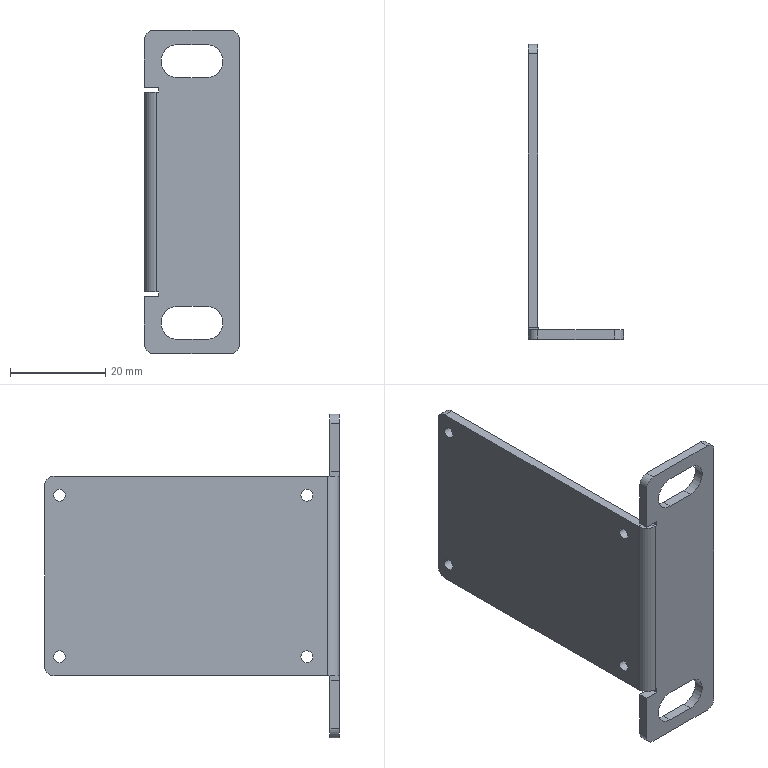Part | SolidWorks | features ICE 4, Cut 1, ExtruThin 1, Fillet 1, FlatPattern 1, FlattenBends 1, ProcessBends 1, SheetMetal 1 | 1 solid | 44 faces | box 20 x 62 x 68 mm | volume 7322 mm3 | plane 24 | cylinder 20 | commonest cylinder face diameters 2.5 x8 4 x6 7 x4 1 x1 5 x1
STEP:
#1=CARTESIAN_POINT('',(0.,8.1,17.));
#2=VERTEX_POINT('',#1);
#3=CARTESIAN_POINT('',(0.,5.6,17.));
#4=VERTEX_POINT('',#3);
#5=CARTESIAN_POINT('',(0.,6.85,17.));
#6=DIRECTION('',(-1.,0.,0.));
#7=DIRECTION('',(0.,-1.,0.));
#8=AXIS2_PLACEMENT_3D('',#5,#6,#7);
#9=CIRCLE('',#8,1.25);
#10=EDGE_CURVE('',#2,#4,#9,.T.);
#11=ORIENTED_EDGE('',*,*,#10,.T.);
#12=CARTESIAN_POINT('',(2.,5.6,17.));
#13=VERTEX_POINT('',#12);
#14=CARTESIAN_POINT('',(-8.,5.6,17.));
#15=DIRECTION('',(1.,0.,0.));
#16=VECTOR('',#15,1000.);
#17=LINE('',#14,#16);
#18=EDGE_CURVE('',#4,#13,#17,.T.);
#19=ORIENTED_EDGE('',*,*,#18,.T.);
#20=CARTESIAN_POINT('',(2.,8.1,17.));
#21=VERTEX_POINT('',#20);
#22=CARTESIAN_POINT('',(2.,6.85,17.));
#23=DIRECTION('',(1.,0.,0.));
#24=DIRECTION('',(0.,1.,0.));
#25=AXIS2_PLACEMENT_3D('',#22,#23,#24);
#26=CIRCLE('',#25,1.25);
#27=EDGE_CURVE('',#13,#21,#26,.T.);
#28=ORIENTED_EDGE('',*,*,#27,.T.);
#29=CARTESIAN_POINT('',(-8.,8.1,17.));
#30=DIRECTION('',(1.,0.,0.));
#31=VECTOR('',#30,1000.);
#32=LINE('',#29,#31);
#33=EDGE_CURVE('',#2,#21,#32,.T.);
#34=ORIENTED_EDGE('',*,*,#33,.F.);
#35=EDGE_LOOP('',(#11,#19,#28,#34));
#36=FACE_OUTER_BOUND('',#35,.T.);
#37=CARTESIAN_POINT('',(-8.,6.85,17.));
#38=DIRECTION('',(1.,0.,0.));
#39=DIRECTION('',(0.,1.,0.));
#40=AXIS2_PLACEMENT_3D('',#37,#38,#39);
#41=CYLINDRICAL_SURFACE('',#40,1.25);
#42=ADVANCED_FACE('',(#36),#41,.F.);
#43=CARTESIAN_POINT('',(0.,8.1,-17.));
#44=VERTEX_POINT('',#43);
#45=CARTESIAN_POINT('',(0.,5.6,-17.));
#46=VERTEX_POINT('',#45);
#47=CARTESIAN_POINT('',(0.,6.85,-17.));
#48=DIRECTION('',(-1.,0.,0.));
#49=DIRECTION('',(0.,-1.,0.));
#50=AXIS2_PLACEMENT_3D('',#47,#48,#49);
#51=CIRCLE('',#50,1.25);
#52=EDGE_CURVE('',#44,#46,#51,.T.);
#53=ORIENTED_EDGE('',*,*,#52,.T.);
#54=CARTESIAN_POINT('',(2.,5.6,-17.));
#55=VERTEX_POINT('',#54);
#56=CARTESIAN_POINT('',(-8.,5.6,-17.));
#57=DIRECTION('',(1.,0.,0.));
#58=VECTOR('',#57,1000.);
#59=LINE('',#56,#58);
#60=EDGE_CURVE('',#46,#55,#59,.T.);
#61=ORIENTED_EDGE('',*,*,#60,.T.);
#62=CARTESIAN_POINT('',(2.,8.1,-17.));
#63=VERTEX_POINT('',#62);
#64=CARTESIAN_POINT('',(2.,6.85,-17.));
#65=DIRECTION('',(1.,0.,0.));
#66=DIRECTION('',(0.,1.,0.));
#67=AXIS2_PLACEMENT_3D('',#64,#65,#66);
#68=CIRCLE('',#67,1.25);
#69=EDGE_CURVE('',#55,#63,#68,.T.);
#70=ORIENTED_EDGE('',*,*,#69,.T.);
#71=CARTESIAN_POINT('',(-8.,8.1,-17.));
#72=DIRECTION('',(1.,0.,0.));
#73=VECTOR('',#72,1000.);
#74=LINE('',#71,#73);
#75=EDGE_CURVE('',#44,#63,#74,.T.);
#76=ORIENTED_EDGE('',*,*,#75,.F.);
#77=EDGE_LOOP('',(#53,#61,#70,#76));
#78=FACE_OUTER_BOUND('',#77,.T.);
#79=CARTESIAN_POINT('',(-8.,6.85,-17.));
#80=DIRECTION('',(1.,0.,0.));
#81=DIRECTION('',(0.,1.,0.));
#82=AXIS2_PLACEMENT_3D('',#79,#80,#81);
#83=CYLINDRICAL_SURFACE('',#82,1.25);
#84=ADVANCED_FACE('',(#78),#83,.F.);
#85=CARTESIAN_POINT('',(0.,60.1,-17.));
#86=VERTEX_POINT('',#85);
#87=CARTESIAN_POINT('',(0.,57.6,-17.));
#88=VERTEX_POINT('',#87);
#89=CARTESIAN_POINT('',(0.,58.85,-17.));
#90=DIRECTION('',(-1.,0.,0.));
#91=DIRECTION('',(0.,-1.,0.));
#92=AXIS2_PLACEMENT_3D('',#89,#90,#91);
#93=CIRCLE('',#92,1.25);
#94=EDGE_CURVE('',#86,#88,#93,.T.);
#95=ORIENTED_EDGE('',*,*,#94,.T.);
#96=CARTESIAN_POINT('',(2.,57.6,-17.));
#97=VERTEX_POINT('',#96);
#98=CARTESIAN_POINT('',(-8.,57.6,-17.));
#99=DIRECTION('',(1.,0.,0.));
#100=VECTOR('',#99,1000.);
#101=LINE('',#98,#100);
#102=EDGE_CURVE('',#88,#97,#101,.T.);
#103=ORIENTED_EDGE('',*,*,#102,.T.);
#104=CARTESIAN_POINT('',(2.,60.1,-17.));
#105=VERTEX_POINT('',#104);
#106=CARTESIAN_POINT('',(2.,58.85,-17.));
#107=DIRECTION('',(1.,0.,0.));
#108=DIRECTION('',(0.,1.,0.));
#109=AXIS2_PLACEMENT_3D('',#106,#107,#108);
#110=CIRCLE('',#109,1.25);
#111=EDGE_CURVE('',#97,#105,#110,.T.);
#112=ORIENTED_EDGE('',*,*,#111,.T.);
#113=CARTESIAN_POINT('',(-8.,60.1,-17.));
#114=DIRECTION('',(1.,0.,0.));
#115=VECTOR('',#114,1000.);
#116=LINE('',#113,#115);
#117=EDGE_CURVE('',#86,#105,#116,.T.);
#118=ORIENTED_EDGE('',*,*,#117,.F.);
#119=EDGE_LOOP('',(#95,#103,#112,#118));
#120=FACE_OUTER_BOUND('',#119,.T.);
#121=CARTESIAN_POINT('',(-8.,58.85,-17.));
#122=DIRECTION('',(1.,0.,0.));
#123=DIRECTION('',(0.,1.,0.));
#124=AXIS2_PLACEMENT_3D('',#121,#122,#123);
#125=CYLINDRICAL_SURFACE('',#124,1.25);
#126=ADVANCED_FACE('',(#120),#125,.F.);
#127=CARTESIAN_POINT('',(0.,60.1,17.));
#128=VERTEX_POINT('',#127);
#129=CARTESIAN_POINT('',(0.,57.6,17.));
#130=VERTEX_POINT('',#129);
#131=CARTESIAN_POINT('',(0.,58.85,17.));
#132=DIRECTION('',(-1.,0.,0.));
#133=DIRECTION('',(0.,-1.,0.));
#134=AXIS2_PLACEMENT_3D('',#131,#132,#133);
#135=CIRCLE('',#134,1.25);
#136=EDGE_CURVE('',#128,#130,#135,.T.);
#137=ORIENTED_EDGE('',*,*,#136,.T.);
#138=CARTESIAN_POINT('',(2.,57.6,17.));
#139=VERTEX_POINT('',#138);
#140=CARTESIAN_POINT('',(-8.,57.6,17.));
#141=DIRECTION('',(1.,0.,0.));
#142=VECTOR('',#141,1000.);
#143=LINE('',#140,#142);
#144=EDGE_CURVE('',#130,#139,#143,.T.);
#145=ORIENTED_EDGE('',*,*,#144,.T.);
#146=CARTESIAN_POINT('',(2.,60.1,17.));
#147=VERTEX_POINT('',#146);
#148=CARTESIAN_POINT('',(2.,58.85,17.));
#149=DIRECTION('',(1.,0.,0.));
#150=DIRECTION('',(0.,1.,0.));
#151=AXIS2_PLACEMENT_3D('',#148,#149,#150);
#152=CIRCLE('',#151,1.25);
#153=EDGE_CURVE('',#139,#147,#152,.T.);
#154=ORIENTED_EDGE('',*,*,#153,.T.);
#155=CARTESIAN_POINT('',(-8.,60.1,17.));
#156=DIRECTION('',(1.,0.,0.));
#157=VECTOR('',#156,1000.);
#158=LINE('',#155,#157);
#159=EDGE_CURVE('',#128,#147,#158,.T.);
#160=ORIENTED_EDGE('',*,*,#159,.F.);
#161=EDGE_LOOP('',(#137,#145,#154,#160));
#162=FACE_OUTER_BOUND('',#161,.T.);
#163=CARTESIAN_POINT('',(-8.,58.85,17.));
#164=DIRECTION('',(1.,0.,0.));
#165=DIRECTION('',(0.,1.,0.));
#166=AXIS2_PLACEMENT_3D('',#163,#164,#165);
#167=CYLINDRICAL_SURFACE('',#166,1.25);
#168=ADVANCED_FACE('',(#162),#167,.F.);
#169=CARTESIAN_POINT('',(7.,0.,-31.));
#170=VERTEX_POINT('',#169);
#171=CARTESIAN_POINT('',(13.,0.,-31.));
#172=VERTEX_POINT('',#171);
#173=CARTESIAN_POINT('',(0.,0.,-31.));
#174=DIRECTION('',(1.,0.,0.));
#175=VECTOR('',#174,1000.);
#176=LINE('',#173,#175);
#177=EDGE_CURVE('',#170,#172,#176,.T.);
#178=ORIENTED_EDGE('',*,*,#177,.T.);
#179=CARTESIAN_POINT('',(13.,2.,-31.));
#180=VERTEX_POINT('',#179);
#181=CARTESIAN_POINT('',(13.,-1.,-31.));
#182=DIRECTION('',(0.,1.,0.));
#183=VECTOR('',#182,1000.);
#184=LINE('',#181,#183);
#185=EDGE_CURVE('',#172,#180,#184,.T.);
#186=ORIENTED_EDGE('',*,*,#185,.T.);
#187=CARTESIAN_POINT('',(7.,2.,-31.));
#188=VERTEX_POINT('',#187);
#189=CARTESIAN_POINT('',(7.,2.,-31.));
#190=DIRECTION('',(-1.,0.,0.));
#191=VECTOR('',#190,1000.);
#192=LINE('',#189,#191);
#193=EDGE_CURVE('',#180,#188,#192,.T.);
#194=ORIENTED_EDGE('',*,*,#193,.T.);
#195=CARTESIAN_POINT('',(7.,-1.,-31.));
#196=DIRECTION('',(0.,1.,0.));
#197=VECTOR('',#196,1000.);
#198=LINE('',#195,#197);
#199=EDGE_CURVE('',#170,#188,#198,.T.);
#200=ORIENTED_EDGE('',*,*,#199,.F.);
#201=EDGE_LOOP('',(#178,#186,#194,#200));
#202=FACE_OUTER_BOUND('',#201,.T.);
#203=CARTESIAN_POINT('',(7.,-1.,-31.));
#204=DIRECTION('',(0.,0.,-1.));
#205=DIRECTION('',(-1.,0.,0.));
#206=AXIS2_PLACEMENT_3D('',#203,#204,#205);
#207=PLANE('',#206);
#208=ADVANCED_FACE('',(#202),#207,.F.);
#209=CARTESIAN_POINT('',(13.,0.,-24.));
#210=VERTEX_POINT('',#209);
#211=CARTESIAN_POINT('',(13.,0.,-27.5));
#212=DIRECTION('',(0.,-1.,0.));
#213=DIRECTION('',(0.,0.,-1.));
#214=AXIS2_PLACEMENT_3D('',#211,#212,#213);
#215=CIRCLE('',#214,3.5);
#216=EDGE_CURVE('',#172,#210,#215,.T.);
#217=ORIENTED_EDGE('',*,*,#216,.T.);
#218=CARTESIAN_POINT('',(13.,2.,-24.));
#219=VERTEX_POINT('',#218);
#220=CARTESIAN_POINT('',(13.,-1.,-24.));
#221=DIRECTION('',(0.,1.,0.));
#222=VECTOR('',#221,1000.);
#223=LINE('',#220,#222);
#224=EDGE_CURVE('',#210,#219,#223,.T.);
#225=ORIENTED_EDGE('',*,*,#224,.T.);
#226=CARTESIAN_POINT('',(13.,2.,-27.5));
#227=DIRECTION('',(0.,1.,0.));
#228=DIRECTION('',(0.,0.,1.));
#229=AXIS2_PLACEMENT_3D('',#226,#227,#228);
#230=CIRCLE('',#229,3.5);
#231=EDGE_CURVE('',#219,#180,#230,.T.);
#232=ORIENTED_EDGE('',*,*,#231,.T.);
#233=ORIENTED_EDGE('',*,*,#185,.F.);
#234=EDGE_LOOP('',(#217,#225,#232,#233));
#235=FACE_OUTER_BOUND('',#234,.T.);
#236=CARTESIAN_POINT('',(13.,-1.,-27.5));
#237=DIRECTION('',(0.,1.,0.));
#238=DIRECTION('',(0.,0.,1.));
#239=AXIS2_PLACEMENT_3D('',#236,#237,#238);
#240=CYLINDRICAL_SURFACE('',#239,3.5);
#241=ADVANCED_FACE('',(#235),#240,.F.);
#242=CARTESIAN_POINT('',(7.,0.,-24.));
#243=VERTEX_POINT('',#242);
#244=CARTESIAN_POINT('',(0.,0.,-24.));
#245=DIRECTION('',(-1.,0.,0.));
#246=VECTOR('',#245,1000.);
#247=LINE('',#244,#246);
#248=EDGE_CURVE('',#210,#243,#247,.T.);
#249=ORIENTED_EDGE('',*,*,#248,.T.);
#250=CARTESIAN_POINT('',(7.,2.,-24.));
#251=VERTEX_POINT('',#250);
#252=CARTESIAN_POINT('',(7.,-1.,-24.));
#253=DIRECTION('',(0.,1.,0.));
#254=VECTOR('',#253,1000.);
#255=LINE('',#252,#254);
#256=EDGE_CURVE('',#243,#251,#255,.T.);
#257=ORIENTED_EDGE('',*,*,#256,.T.);
#258=CARTESIAN_POINT('',(7.,2.,-24.));
#259=DIRECTION('',(1.,0.,0.));
#260=VECTOR('',#259,1000.);
#261=LINE('',#258,#260);
#262=EDGE_CURVE('',#251,#219,#261,.T.);
#263=ORIENTED_EDGE('',*,*,#262,.T.);
#264=ORIENTED_EDGE('',*,*,#224,.F.);
#265=EDGE_LOOP('',(#249,#257,#263,#264));
#266=FACE_OUTER_BOUND('',#265,.T.);
#267=CARTESIAN_POINT('',(7.,-1.,-24.));
#268=DIRECTION('',(0.,0.,1.));
#269=DIRECTION('',(1.,0.,0.));
#270=AXIS2_PLACEMENT_3D('',#267,#268,#269);
#271=PLANE('',#270);
#272=ADVANCED_FACE('',(#266),#271,.F.);
#273=CARTESIAN_POINT('',(7.,0.,-27.5));
#274=DIRECTION('',(0.,-1.,0.));
#275=DIRECTION('',(0.,0.,-1.));
#276=AXIS2_PLACEMENT_3D('',#273,#274,#275);
#277=CIRCLE('',#276,3.5);
#278=EDGE_CURVE('',#243,#170,#277,.T.);
#279=ORIENTED_EDGE('',*,*,#278,.T.);
#280=ORIENTED_EDGE('',*,*,#199,.T.);
#281=CARTESIAN_POINT('',(7.,2.,-27.5));
#282=DIRECTION('',(0.,1.,0.));
#283=DIRECTION('',(0.,0.,1.));
#284=AXIS2_PLACEMENT_3D('',#281,#282,#283);
#285=CIRCLE('',#284,3.5);
#286=EDGE_CURVE('',#188,#251,#285,.T.);
#287=ORIENTED_EDGE('',*,*,#286,.T.);
#288=ORIENTED_EDGE('',*,*,#256,.F.);
#289=EDGE_LOOP('',(#279,#280,#287,#288));
#290=FACE_OUTER_BOUND('',#289,.T.);
#291=CARTESIAN_POINT('',(7.,-1.,-27.5));
#292=DIRECTION('',(0.,1.,0.));
#293=DIRECTION('',(0.,0.,1.));
#294=AXIS2_PLACEMENT_3D('',#291,#292,#293);
#295=CYLINDRICAL_SURFACE('',#294,3.5);
#296=ADVANCED_FACE('',(#290),#295,.F.);
#297=CARTESIAN_POINT('',(7.,0.,24.));
#298=VERTEX_POINT('',#297);
#299=CARTESIAN_POINT('',(13.,0.,24.));
#300=VERTEX_POINT('',#299);
#301=CARTESIAN_POINT('',(0.,0.,24.));
#302=DIRECTION('',(1.,0.,0.));
#303=VECTOR('',#302,1000.);
#304=LINE('',#301,#303);
#305=EDGE_CURVE('',#298,#300,#304,.T.);
#306=ORIENTED_EDGE('',*,*,#305,.T.);
#307=CARTESIAN_POINT('',(13.,2.,24.));
#308=VERTEX_POINT('',#307);
#309=CARTESIAN_POINT('',(13.,-1.,24.));
#310=DIRECTION('',(0.,1.,0.));
#311=VECTOR('',#310,1000.);
#312=LINE('',#309,#311);
#313=EDGE_CURVE('',#300,#308,#312,.T.);
#314=ORIENTED_EDGE('',*,*,#313,.T.);
#315=CARTESIAN_POINT('',(7.,2.,24.));
#316=VERTEX_POINT('',#315);
#317=CARTESIAN_POINT('',(7.,2.,24.));
#318=DIRECTION('',(-1.,0.,0.));
#319=VECTOR('',#318,1000.);
#320=LINE('',#317,#319);
#321=EDGE_CURVE('',#308,#316,#320,.T.);
#322=ORIENTED_EDGE('',*,*,#321,.T.);
#323=CARTESIAN_POINT('',(7.,-1.,24.));
#324=DIRECTION('',(0.,1.,0.));
#325=VECTOR('',#324,1000.);
#326=LINE('',#323,#325);
#327=EDGE_CURVE('',#298,#316,#326,.T.);
#328=ORIENTED_EDGE('',*,*,#327,.F.);
#329=EDGE_LOOP('',(#306,#314,#322,#328));
#330=FACE_OUTER_BOUND('',#329,.T.);
#331=CARTESIAN_POINT('',(7.,-1.,24.));
#332=DIRECTION('',(0.,0.,-1.));
#333=DIRECTION('',(-1.,0.,0.));
#334=AXIS2_PLACEMENT_3D('',#331,#332,#333);
#335=PLANE('',#334);
#336=ADVANCED_FACE('',(#330),#335,.F.);
#337=CARTESIAN_POINT('',(13.,0.,31.));
#338=VERTEX_POINT('',#337);
#339=CARTESIAN_POINT('',(13.,0.,27.5));
#340=DIRECTION('',(0.,-1.,0.));
#341=DIRECTION('',(0.,0.,-1.));
#342=AXIS2_PLACEMENT_3D('',#339,#340,#341);
#343=CIRCLE('',#342,3.5);
#344=EDGE_CURVE('',#300,#338,#343,.T.);
#345=ORIENTED_EDGE('',*,*,#344,.T.);
#346=CARTESIAN_POINT('',(13.,2.,31.));
#347=VERTEX_POINT('',#346);
#348=CARTESIAN_POINT('',(13.,-1.,31.));
#349=DIRECTION('',(0.,1.,0.));
#350=VECTOR('',#349,1000.);
#351=LINE('',#348,#350);
#352=EDGE_CURVE('',#338,#347,#351,.T.);
#353=ORIENTED_EDGE('',*,*,#352,.T.);
#354=CARTESIAN_POINT('',(13.,2.,27.5));
#355=DIRECTION('',(0.,1.,0.));
#356=DIRECTION('',(0.,0.,1.));
#357=AXIS2_PLACEMENT_3D('',#354,#355,#356);
#358=CIRCLE('',#357,3.5);
#359=EDGE_CURVE('',#347,#308,#358,.T.);
#360=ORIENTED_EDGE('',*,*,#359,.T.);
#361=ORIENTED_EDGE('',*,*,#313,.F.);
#362=EDGE_LOOP('',(#345,#353,#360,#361));
#363=FACE_OUTER_BOUND('',#362,.T.);
#364=CARTESIAN_POINT('',(13.,-1.,27.5));
#365=DIRECTION('',(0.,1.,0.));
#366=DIRECTION('',(0.,0.,1.));
#367=AXIS2_PLACEMENT_3D('',#364,#365,#366);
#368=CYLINDRICAL_SURFACE('',#367,3.5);
#369=ADVANCED_FACE('',(#363),#368,.F.);
#370=CARTESIAN_POINT('',(7.,0.,31.));
#371=VERTEX_POINT('',#370);
#372=CARTESIAN_POINT('',(0.,0.,31.));
#373=DIRECTION('',(-1.,0.,0.));
#374=VECTOR('',#373,1000.);
#375=LINE('',#372,#374);
#376=EDGE_CURVE('',#338,#371,#375,.T.);
#377=ORIENTED_EDGE('',*,*,#376,.T.);
#378=CARTESIAN_POINT('',(7.,2.,31.));
#379=VERTEX_POINT('',#378);
#380=CARTESIAN_POINT('',(7.,-1.,31.));
#381=DIRECTION('',(0.,1.,0.));
#382=VECTOR('',#381,1000.);
#383=LINE('',#380,#382);
#384=EDGE_CURVE('',#371,#379,#383,.T.);
#385=ORIENTED_EDGE('',*,*,#384,.T.);
#386=CARTESIAN_POINT('',(7.,2.,31.));
#387=DIRECTION('',(1.,0.,0.));
#388=VECTOR('',#387,1000.);
#389=LINE('',#386,#388);
#390=EDGE_CURVE('',#379,#347,#389,.T.);
#391=ORIENTED_EDGE('',*,*,#390,.T.);
#392=ORIENTED_EDGE('',*,*,#352,.F.);
#393=EDGE_LOOP('',(#377,#385,#391,#392));
#394=FACE_OUTER_BOUND('',#393,.T.);
#395=CARTESIAN_POINT('',(7.,-1.,31.));
#396=DIRECTION('',(0.,0.,1.));
#397=DIRECTION('',(1.,0.,0.));
#398=AXIS2_PLACEMENT_3D('',#395,#396,#397);
#399=PLANE('',#398);
#400=ADVANCED_FACE('',(#394),#399,.F.);
#401=CARTESIAN_POINT('',(7.,0.,27.5));
#402=DIRECTION('',(0.,-1.,0.));
#403=DIRECTION('',(0.,0.,-1.));
#404=AXIS2_PLACEMENT_3D('',#401,#402,#403);
#405=CIRCLE('',#404,3.5);
#406=EDGE_CURVE('',#371,#298,#405,.T.);
#407=ORIENTED_EDGE('',*,*,#406,.T.);
#408=ORIENTED_EDGE('',*,*,#327,.T.);
#409=CARTESIAN_POINT('',(7.,2.,27.5));
#410=DIRECTION('',(0.,1.,0.));
#411=DIRECTION('',(0.,0.,1.));
#412=AXIS2_PLACEMENT_3D('',#409,#410,#411);
#413=CIRCLE('',#412,3.5);
#414=EDGE_CURVE('',#316,#379,#413,.T.);
#415=ORIENTED_EDGE('',*,*,#414,.T.);
#416=ORIENTED_EDGE('',*,*,#384,.F.);
#417=EDGE_LOOP('',(#407,#408,#415,#416));
#418=FACE_OUTER_BOUND('',#417,.T.);
#419=CARTESIAN_POINT('',(7.,-1.,27.5));
#420=DIRECTION('',(0.,1.,0.));
#421=DIRECTION('',(0.,0.,1.));
#422=AXIS2_PLACEMENT_3D('',#419,#420,#421);
#423=CYLINDRICAL_SURFACE('',#422,3.5);
#424=ADVANCED_FACE('',(#418),#423,.F.);
#425=CARTESIAN_POINT('',(3.,0.,22.));
#426=VERTEX_POINT('',#425);
#427=CARTESIAN_POINT('',(0.,0.,22.));
#428=VERTEX_POINT('',#427);
#429=CARTESIAN_POINT('',(0.,0.,22.));
#430=DIRECTION('',(-1.,0.,0.));
#431=VECTOR('',#430,1000.);
#432=LINE('',#429,#431);
#433=EDGE_CURVE('',#426,#428,#432,.T.);
#434=ORIENTED_EDGE('',*,*,#433,.T.);
#435=CARTESIAN_POINT('',(0.,2.,22.));
#436=VERTEX_POINT('',#435);
#437=CARTESIAN_POINT('',(0.,141.76,22.));
#438=DIRECTION('',(0.,-1.,0.));
#439=VECTOR('',#438,1000.);
#440=LINE('',#437,#439);
#441=EDGE_CURVE('',#436,#428,#440,.T.);
#442=ORIENTED_EDGE('',*,*,#441,.F.);
#443=CARTESIAN_POINT('',(3.,2.,22.));
#444=VERTEX_POINT('',#443);
#445=CARTESIAN_POINT('',(3.,2.,22.));
#446=DIRECTION('',(-1.,0.,0.));
#447=VECTOR('',#446,1000.);
#448=LINE('',#445,#447);
#449=EDGE_CURVE('',#444,#436,#448,.T.);
#450=ORIENTED_EDGE('',*,*,#449,.F.);
#451=CARTESIAN_POINT('',(3.,141.76,22.));
#452=DIRECTION('',(0.,-1.,0.));
#453=VECTOR('',#452,1000.);
#454=LINE('',#451,#453);
#455=EDGE_CURVE('',#444,#426,#454,.T.);
#456=ORIENTED_EDGE('',*,*,#455,.T.);
#457=EDGE_LOOP('',(#434,#442,#450,#456));
#458=FACE_OUTER_BOUND('',#457,.T.);
#459=CARTESIAN_POINT('',(3.,141.76,22.));
#460=DIRECTION('',(0.,0.,1.));
#461=DIRECTION('',(0.,1.,0.));
#462=AXIS2_PLACEMENT_3D('',#459,#460,#461);
#463=PLANE('',#462);
#464=ADVANCED_FACE('',(#458),#463,.F.);
#465=CARTESIAN_POINT('',(0.,0.,32.));
#466=VERTEX_POINT('',#465);
#467=CARTESIAN_POINT('',(0.,0.,-34.));
#468=DIRECTION('',(0.,0.,1.));
#469=VECTOR('',#468,1000.);
#470=LINE('',#467,#469);
#471=EDGE_CURVE('',#428,#466,#470,.T.);
#472=ORIENTED_EDGE('',*,*,#471,.T.);
#473=CARTESIAN_POINT('',(0.,2.,32.));
#474=VERTEX_POINT('',#473);
#475=CARTESIAN_POINT('',(0.,141.76,32.));
#476=DIRECTION('',(0.,-1.,0.));
#477=VECTOR('',#476,1000.);
#478=LINE('',#475,#477);
#479=EDGE_CURVE('',#474,#466,#478,.T.);
#480=ORIENTED_EDGE('',*,*,#479,.F.);
#481=CARTESIAN_POINT('',(0.,2.,34.));
#482=DIRECTION('',(0.,0.,1.));
#483=VECTOR('',#482,1000.);
#484=LINE('',#481,#483);
#485=EDGE_CURVE('',#436,#474,#484,.T.);
#486=ORIENTED_EDGE('',*,*,#485,.F.);
#487=ORIENTED_EDGE('',*,*,#441,.T.);
#488=EDGE_LOOP('',(#472,#480,#486,#487));
#489=FACE_OUTER_BOUND('',#488,.T.);
#490=CARTESIAN_POINT('',(0.,141.76,34.));
#491=DIRECTION('',(1.,0.,0.));
#492=DIRECTION('',(0.,1.,0.));
#493=AXIS2_PLACEMENT_3D('',#490,#491,#492);
#494=PLANE('',#493);
#495=ADVANCED_FACE('',(#489),#494,.F.);
#496=CARTESIAN_POINT('',(2.,0.,34.));
#497=VERTEX_POINT('',#496);
#498=CARTESIAN_POINT('',(2.,0.,32.));
#499=DIRECTION('',(0.,-1.,0.));
#500=DIRECTION('',(0.,0.,-1.));
#501=AXIS2_PLACEMENT_3D('',#498,#499,#500);
#502=CIRCLE('',#501,2.);
#503=EDGE_CURVE('',#497,#466,#502,.T.);
#504=ORIENTED_EDGE('',*,*,#503,.F.);
#505=CARTESIAN_POINT('',(2.,2.,34.));
#506=VERTEX_POINT('',#505);
#507=CARTESIAN_POINT('',(2.,141.76,34.));
#508=DIRECTION('',(0.,-1.,0.));
#509=VECTOR('',#508,1000.);
#510=LINE('',#507,#509);
#511=EDGE_CURVE('',#506,#497,#510,.T.);
#512=ORIENTED_EDGE('',*,*,#511,.F.);
#513=CARTESIAN_POINT('',(2.,2.,32.));
#514=DIRECTION('',(0.,1.,0.));
#515=DIRECTION('',(0.,0.,-1.));
#516=AXIS2_PLACEMENT_3D('',#513,#514,#515);
#517=CIRCLE('',#516,2.);
#518=EDGE_CURVE('',#474,#506,#517,.T.);
#519=ORIENTED_EDGE('',*,*,#518,.F.);
#520=ORIENTED_EDGE('',*,*,#479,.T.);
#521=EDGE_LOOP('',(#504,#512,#519,#520));
#522=FACE_OUTER_BOUND('',#521,.T.);
#523=CARTESIAN_POINT('',(2.,141.76,32.));
#524=DIRECTION('',(0.,-1.,0.));
#525=DIRECTION('',(1.,0.,0.));
#526=AXIS2_PLACEMENT_3D('',#523,#524,#525);
#527=CYLINDRICAL_SURFACE('',#526,2.);
#528=ADVANCED_FACE('',(#522),#527,.T.);
#529=CARTESIAN_POINT('',(18.,0.,34.));
#530=VERTEX_POINT('',#529);
#531=CARTESIAN_POINT('',(0.,0.,34.));
#532=DIRECTION('',(1.,0.,0.));
#533=VECTOR('',#532,1000.);
#534=LINE('',#531,#533);
#535=EDGE_CURVE('',#497,#530,#534,.T.);
#536=ORIENTED_EDGE('',*,*,#535,.T.);
#537=CARTESIAN_POINT('',(18.,2.,34.));
#538=VERTEX_POINT('',#537);
#539=CARTESIAN_POINT('',(18.,141.76,34.));
#540=DIRECTION('',(0.,-1.,0.));
#541=VECTOR('',#540,1000.);
#542=LINE('',#539,#541);
#543=EDGE_CURVE('',#538,#530,#542,.T.);
#544=ORIENTED_EDGE('',*,*,#543,.F.);
#545=CARTESIAN_POINT('',(0.,2.,34.));
#546=DIRECTION('',(1.,0.,0.));
#547=VECTOR('',#546,1000.);
#548=LINE('',#545,#547);
#549=EDGE_CURVE('',#506,#538,#548,.T.);
#550=ORIENTED_EDGE('',*,*,#549,.F.);
#551=ORIENTED_EDGE('',*,*,#511,.T.);
#552=EDGE_LOOP('',(#536,#544,#550,#551));
#553=FACE_OUTER_BOUND('',#552,.T.);
#554=CARTESIAN_POINT('',(0.,141.76,34.));
#555=DIRECTION('',(0.,0.,-1.));
#556=DIRECTION('',(0.,-1.,0.));
#557=AXIS2_PLACEMENT_3D('',#554,#555,#556);
#558=PLANE('',#557);
#559=ADVANCED_FACE('',(#553),#558,.F.);
#560=CARTESIAN_POINT('',(20.,0.,32.));
#561=VERTEX_POINT('',#560);
#562=CARTESIAN_POINT('',(18.,0.,32.));
#563=DIRECTION('',(0.,-1.,0.));
#564=DIRECTION('',(0.,0.,-1.));
#565=AXIS2_PLACEMENT_3D('',#562,#563,#564);
#566=CIRCLE('',#565,2.);
#567=EDGE_CURVE('',#561,#530,#566,.T.);
#568=ORIENTED_EDGE('',*,*,#567,.F.);
#569=CARTESIAN_POINT('',(20.,2.,32.));
#570=VERTEX_POINT('',#569);
#571=CARTESIAN_POINT('',(20.,141.76,32.));
#572=DIRECTION('',(0.,-1.,0.));
#573=VECTOR('',#572,1000.);
#574=LINE('',#571,#573);
#575=EDGE_CURVE('',#570,#561,#574,.T.);
#576=ORIENTED_EDGE('',*,*,#575,.F.);
#577=CARTESIAN_POINT('',(18.,2.,32.));
#578=DIRECTION('',(0.,1.,0.));
#579=DIRECTION('',(0.,0.,-1.));
#580=AXIS2_PLACEMENT_3D('',#577,#578,#579);
#581=CIRCLE('',#580,2.);
#582=EDGE_CURVE('',#538,#570,#581,.T.);
#583=ORIENTED_EDGE('',*,*,#582,.F.);
#584=ORIENTED_EDGE('',*,*,#543,.T.);
#585=EDGE_LOOP('',(#568,#576,#583,#584));
#586=FACE_OUTER_BOUND('',#585,.T.);
#587=CARTESIAN_POINT('',(18.,141.76,32.));
#588=DIRECTION('',(0.,-1.,0.));
#589=DIRECTION('',(1.,0.,0.));
#590=AXIS2_PLACEMENT_3D('',#587,#588,#589);
#591=CYLINDRICAL_SURFACE('',#590,2.);
#592=ADVANCED_FACE('',(#586),#591,.T.);
#593=ORIENTED_EDGE('',*,*,#575,.T.);
#594=CARTESIAN_POINT('',(20.,0.,-32.));
#595=VERTEX_POINT('',#594);
#596=CARTESIAN_POINT('',(20.,0.,-34.));
#597=DIRECTION('',(0.,0.,1.));
#598=VECTOR('',#597,1000.);
#599=LINE('',#596,#598);
#600=EDGE_CURVE('',#595,#561,#599,.T.);
#601=ORIENTED_EDGE('',*,*,#600,.F.);
#602=CARTESIAN_POINT('',(20.,2.,-32.));
#603=VERTEX_POINT('',#602);
#604=CARTESIAN_POINT('',(20.,141.76,-32.));
#605=DIRECTION('',(0.,-1.,0.));
#606=VECTOR('',#605,1000.);
#607=LINE('',#604,#606);
#608=EDGE_CURVE('',#603,#595,#607,.T.);
#609=ORIENTED_EDGE('',*,*,#608,.F.);
#610=CARTESIAN_POINT('',(20.,2.,-34.));
#611=DIRECTION('',(0.,0.,1.));
#612=VECTOR('',#611,1000.);
#613=LINE('',#610,#612);
#614=EDGE_CURVE('',#603,#570,#613,.T.);
#615=ORIENTED_EDGE('',*,*,#614,.T.);
#616=EDGE_LOOP('',(#593,#601,#609,#615));
#617=FACE_OUTER_BOUND('',#616,.T.);
#618=CARTESIAN_POINT('',(20.,141.76,-34.));
#619=DIRECTION('',(1.,0.,0.));
#620=DIRECTION('',(0.,1.,0.));
#621=AXIS2_PLACEMENT_3D('',#618,#619,#620);
#622=PLANE('',#621);
#623=ADVANCED_FACE('',(#617),#622,.T.);
#624=CARTESIAN_POINT('',(18.,0.,-34.));
#625=VERTEX_POINT('',#624);
#626=CARTESIAN_POINT('',(18.,0.,-32.));
#627=DIRECTION('',(0.,-1.,0.));
#628=DIRECTION('',(0.,0.,-1.));
#629=AXIS2_PLACEMENT_3D('',#626,#627,#628);
#630=CIRCLE('',#629,2.);
#631=EDGE_CURVE('',#625,#595,#630,.T.);
#632=ORIENTED_EDGE('',*,*,#631,.F.);
#633=CARTESIAN_POINT('',(18.,2.,-34.));
#634=VERTEX_POINT('',#633);
#635=CARTESIAN_POINT('',(18.,141.76,-34.));
#636=DIRECTION('',(0.,-1.,0.));
#637=VECTOR('',#636,1000.);
#638=LINE('',#635,#637);
#639=EDGE_CURVE('',#634,#625,#638,.T.);
#640=ORIENTED_EDGE('',*,*,#639,.F.);
#641=CARTESIAN_POINT('',(18.,2.,-32.));
#642=DIRECTION('',(0.,1.,0.));
#643=DIRECTION('',(0.,0.,-1.));
#644=AXIS2_PLACEMENT_3D('',#641,#642,#643);
#645=CIRCLE('',#644,2.);
#646=EDGE_CURVE('',#603,#634,#645,.T.);
#647=ORIENTED_EDGE('',*,*,#646,.F.);
#648=ORIENTED_EDGE('',*,*,#608,.T.);
#649=EDGE_LOOP('',(#632,#640,#647,#648));
#650=FACE_OUTER_BOUND('',#649,.T.);
#651=CARTESIAN_POINT('',(18.,141.76,-32.));
#652=DIRECTION('',(0.,-1.,0.));
#653=DIRECTION('',(1.,0.,0.));
#654=AXIS2_PLACEMENT_3D('',#651,#652,#653);
#655=CYLINDRICAL_SURFACE('',#654,2.);
#656=ADVANCED_FACE('',(#650),#655,.T.);
#657=ORIENTED_EDGE('',*,*,#639,.T.);
#658=CARTESIAN_POINT('',(2.,0.,-34.));
#659=VERTEX_POINT('',#658);
#660=CARTESIAN_POINT('',(0.,0.,-34.));
#661=DIRECTION('',(1.,0.,0.));
#662=VECTOR('',#661,1000.);
#663=LINE('',#660,#662);
#664=EDGE_CURVE('',#659,#625,#663,.T.);
#665=ORIENTED_EDGE('',*,*,#664,.F.);
#666=CARTESIAN_POINT('',(2.,2.,-34.));
#667=VERTEX_POINT('',#666);
#668=CARTESIAN_POINT('',(2.,141.76,-34.));
#669=DIRECTION('',(0.,-1.,0.));
#670=VECTOR('',#669,1000.);
#671=LINE('',#668,#670);
#672=EDGE_CURVE('',#667,#659,#671,.T.);
#673=ORIENTED_EDGE('',*,*,#672,.F.);
#674=CARTESIAN_POINT('',(0.,2.,-34.));
#675=DIRECTION('',(1.,0.,0.));
#676=VECTOR('',#675,1000.);
#677=LINE('',#674,#676);
#678=EDGE_CURVE('',#667,#634,#677,.T.);
#679=ORIENTED_EDGE('',*,*,#678,.T.);
#680=EDGE_LOOP('',(#657,#665,#673,#679));
#681=FACE_OUTER_BOUND('',#680,.T.);
#682=CARTESIAN_POINT('',(0.,141.76,-34.));
#683=DIRECTION('',(0.,0.,-1.));
#684=DIRECTION('',(0.,-1.,0.));
#685=AXIS2_PLACEMENT_3D('',#682,#683,#684);
#686=PLANE('',#685);
#687=ADVANCED_FACE('',(#681),#686,.T.);
#688=CARTESIAN_POINT('',(0.,0.,-32.));
#689=VERTEX_POINT('',#688);
#690=CARTESIAN_POINT('',(2.,0.,-32.));
#691=DIRECTION('',(0.,-1.,0.));
#692=DIRECTION('',(0.,0.,-1.));
#693=AXIS2_PLACEMENT_3D('',#690,#691,#692);
#694=CIRCLE('',#693,2.);
#695=EDGE_CURVE('',#689,#659,#694,.T.);
#696=ORIENTED_EDGE('',*,*,#695,.F.);
#697=CARTESIAN_POINT('',(0.,2.,-32.));
#698=VERTEX_POINT('',#697);
#699=CARTESIAN_POINT('',(0.,141.76,-32.));
#700=DIRECTION('',(0.,-1.,0.));
#701=VECTOR('',#700,1000.);
#702=LINE('',#699,#701);
#703=EDGE_CURVE('',#698,#689,#702,.T.);
#704=ORIENTED_EDGE('',*,*,#703,.F.);
#705=CARTESIAN_POINT('',(2.,2.,-32.));
#706=DIRECTION('',(0.,1.,0.));
#707=DIRECTION('',(0.,0.,-1.));
#708=AXIS2_PLACEMENT_3D('',#705,#706,#707);
#709=CIRCLE('',#708,2.);
#710=EDGE_CURVE('',#667,#698,#709,.T.);
#711=ORIENTED_EDGE('',*,*,#710,.F.);
#712=ORIENTED_EDGE('',*,*,#672,.T.);
#713=EDGE_LOOP('',(#696,#704,#711,#712));
#714=FACE_OUTER_BOUND('',#713,.T.);
#715=CARTESIAN_POINT('',(2.,141.76,-32.));
#716=DIRECTION('',(0.,-1.,0.));
#717=DIRECTION('',(1.,0.,0.));
#718=AXIS2_PLACEMENT_3D('',#715,#716,#717);
#719=CYLINDRICAL_SURFACE('',#718,2.);
#720=ADVANCED_FACE('',(#714),#719,.T.);
#721=CARTESIAN_POINT('',(0.,0.,-22.));
#722=VERTEX_POINT('',#721);
#723=CARTESIAN_POINT('',(0.,0.,-34.));
#724=DIRECTION('',(0.,0.,1.));
#725=VECTOR('',#724,1000.);
#726=LINE('',#723,#725);
#727=EDGE_CURVE('',#689,#722,#726,.T.);
#728=ORIENTED_EDGE('',*,*,#727,.T.);
#729=CARTESIAN_POINT('',(0.,2.,-22.));
#730=VERTEX_POINT('',#729);
#731=CARTESIAN_POINT('',(0.,141.76,-22.));
#732=DIRECTION('',(0.,-1.,0.));
#733=VECTOR('',#732,1000.);
#734=LINE('',#731,#733);
#735=EDGE_CURVE('',#730,#722,#734,.T.);
#736=ORIENTED_EDGE('',*,*,#735,.F.);
#737=CARTESIAN_POINT('',(0.,2.,-34.));
#738=DIRECTION('',(0.,0.,1.));
#739=VECTOR('',#738,1000.);
#740=LINE('',#737,#739);
#741=EDGE_CURVE('',#698,#730,#740,.T.);
#742=ORIENTED_EDGE('',*,*,#741,.F.);
#743=ORIENTED_EDGE('',*,*,#703,.T.);
#744=EDGE_LOOP('',(#728,#736,#742,#743));
#745=FACE_OUTER_BOUND('',#744,.T.);
#746=CARTESIAN_POINT('',(0.,141.76,-34.));
#747=DIRECTION('',(1.,0.,0.));
#748=DIRECTION('',(0.,1.,0.));
#749=AXIS2_PLACEMENT_3D('',#746,#747,#748);
#750=PLANE('',#749);
#751=ADVANCED_FACE('',(#745),#750,.F.);
#752=ORIENTED_EDGE('',*,*,#735,.T.);
#753=CARTESIAN_POINT('',(3.,0.,-22.));
#754=VERTEX_POINT('',#753);
#755=CARTESIAN_POINT('',(0.,0.,-22.));
#756=DIRECTION('',(1.,0.,0.));
#757=VECTOR('',#756,1000.);
#758=LINE('',#755,#757);
#759=EDGE_CURVE('',#722,#754,#758,.T.);
#760=ORIENTED_EDGE('',*,*,#759,.T.);
#761=CARTESIAN_POINT('',(3.,2.,-22.));
#762=VERTEX_POINT('',#761);
#763=CARTESIAN_POINT('',(3.,141.76,-22.));
#764=DIRECTION('',(0.,-1.,0.));
#765=VECTOR('',#764,1000.);
#766=LINE('',#763,#765);
#767=EDGE_CURVE('',#762,#754,#766,.T.);
#768=ORIENTED_EDGE('',*,*,#767,.F.);
#769=CARTESIAN_POINT('',(3.,2.,-22.));
#770=DIRECTION('',(-1.,0.,0.));
#771=VECTOR('',#770,1000.);
#772=LINE('',#769,#771);
#773=EDGE_CURVE('',#762,#730,#772,.T.);
#774=ORIENTED_EDGE('',*,*,#773,.T.);
#775=EDGE_LOOP('',(#752,#760,#768,#774));
#776=FACE_OUTER_BOUND('',#775,.T.);
#777=CARTESIAN_POINT('',(3.,141.76,-22.));
#778=DIRECTION('',(0.,0.,1.));
#779=DIRECTION('',(0.,1.,0.));
#780=AXIS2_PLACEMENT_3D('',#777,#778,#779);
#781=PLANE('',#780);
#782=ADVANCED_FACE('',(#776),#781,.T.);
#783=ORIENTED_EDGE('',*,*,#767,.T.);
#784=CARTESIAN_POINT('',(3.,0.,-21.));
#785=VERTEX_POINT('',#784);
#786=CARTESIAN_POINT('',(3.,0.,-34.));
#787=DIRECTION('',(0.,0.,1.));
#788=VECTOR('',#787,1000.);
#789=LINE('',#786,#788);
#790=EDGE_CURVE('',#754,#785,#789,.T.);
#791=ORIENTED_EDGE('',*,*,#790,.T.);
#792=CARTESIAN_POINT('',(3.,2.,-21.));
#793=VERTEX_POINT('',#792);
#794=CARTESIAN_POINT('',(3.,141.76,-21.));
#795=DIRECTION('',(0.,-1.,0.));
#796=VECTOR('',#795,1000.);
#797=LINE('',#794,#796);
#798=EDGE_CURVE('',#793,#785,#797,.T.);
#799=ORIENTED_EDGE('',*,*,#798,.F.);
#800=CARTESIAN_POINT('',(3.,2.,-21.));
#801=DIRECTION('',(0.,0.,-1.));
#802=VECTOR('',#801,1000.);
#803=LINE('',#800,#802);
#804=EDGE_CURVE('',#793,#762,#803,.T.);
#805=ORIENTED_EDGE('',*,*,#804,.T.);
#806=EDGE_LOOP('',(#783,#791,#799,#805));
#807=FACE_OUTER_BOUND('',#806,.T.);
#808=CARTESIAN_POINT('',(3.,141.76,-21.));
#809=DIRECTION('',(-1.,0.,0.));
#810=DIRECTION('',(0.,-1.,0.));
#811=AXIS2_PLACEMENT_3D('',#808,#809,#810);
#812=PLANE('',#811);
#813=ADVANCED_FACE('',(#807),#812,.T.);
#814=CARTESIAN_POINT('',(3.,2.,21.));
#815=VERTEX_POINT('',#814);
#816=CARTESIAN_POINT('',(3.,0.,21.));
#817=VERTEX_POINT('',#816);
#818=CARTESIAN_POINT('',(3.,141.76,21.));
#819=DIRECTION('',(0.,-1.,0.));
#820=VECTOR('',#819,1000.);
#821=LINE('',#818,#820);
#822=EDGE_CURVE('',#815,#817,#821,.T.);
#823=ORIENTED_EDGE('',*,*,#822,.T.);
#824=CARTESIAN_POINT('',(3.,0.,-34.));
#825=DIRECTION('',(0.,0.,-1.));
#826=VECTOR('',#825,1000.);
#827=LINE('',#824,#826);
#828=EDGE_CURVE('',#426,#817,#827,.T.);
#829=ORIENTED_EDGE('',*,*,#828,.F.);
#830=ORIENTED_EDGE('',*,*,#455,.F.);
#831=CARTESIAN_POINT('',(3.,2.,21.));
#832=DIRECTION('',(0.,0.,-1.));
#833=VECTOR('',#832,1000.);
#834=LINE('',#831,#833);
#835=EDGE_CURVE('',#444,#815,#834,.T.);
#836=ORIENTED_EDGE('',*,*,#835,.T.);
#837=EDGE_LOOP('',(#823,#829,#830,#836));
#838=FACE_OUTER_BOUND('',#837,.T.);
#839=CARTESIAN_POINT('',(3.,141.76,21.));
#840=DIRECTION('',(-1.,0.,0.));
#841=DIRECTION('',(0.,-1.,0.));
#842=AXIS2_PLACEMENT_3D('',#839,#840,#841);
#843=PLANE('',#842);
#844=ADVANCED_FACE('',(#838),#843,.T.);
#845=CARTESIAN_POINT('',(2.5,2.,21.));
#846=VERTEX_POINT('',#845);
#847=CARTESIAN_POINT('',(2.5,0.,21.));
#848=VERTEX_POINT('',#847);
#849=CARTESIAN_POINT('',(2.5,141.76,21.));
#850=DIRECTION('',(0.,-1.,0.));
#851=VECTOR('',#850,1000.);
#852=LINE('',#849,#851);
#853=EDGE_CURVE('',#846,#848,#852,.T.);
#854=ORIENTED_EDGE('',*,*,#853,.T.);
#855=CARTESIAN_POINT('',(0.,0.,21.));
#856=DIRECTION('',(1.,0.,0.));
#857=VECTOR('',#856,1000.);
#858=LINE('',#855,#857);
#859=EDGE_CURVE('',#848,#817,#858,.T.);
#860=ORIENTED_EDGE('',*,*,#859,.T.);
#861=ORIENTED_EDGE('',*,*,#822,.F.);
#862=CARTESIAN_POINT('',(3.,2.,21.));
#863=DIRECTION('',(-1.,0.,0.));
#864=VECTOR('',#863,1000.);
#865=LINE('',#862,#864);
#866=EDGE_CURVE('',#815,#846,#865,.T.);
#867=ORIENTED_EDGE('',*,*,#866,.T.);
#868=EDGE_LOOP('',(#854,#860,#861,#867));
#869=FACE_OUTER_BOUND('',#868,.T.);
#870=CARTESIAN_POINT('',(3.,141.76,21.));
#871=DIRECTION('',(0.,0.,1.));
#872=DIRECTION('',(0.,1.,0.));
#873=AXIS2_PLACEMENT_3D('',#870,#871,#872);
#874=PLANE('',#873);
#875=ADVANCED_FACE('',(#869),#874,.T.);
#876=CARTESIAN_POINT('',(2.5,0.,-21.));
#877=VERTEX_POINT('',#876);
#878=CARTESIAN_POINT('',(2.5,0.,21.));
#879=DIRECTION('',(0.,0.,1.));
#880=VECTOR('',#879,1000.);
#881=LINE('',#878,#880);
#882=EDGE_CURVE('',#877,#848,#881,.T.);
#883=ORIENTED_EDGE('',*,*,#882,.F.);
#884=CARTESIAN_POINT('',(0.,0.,-21.));
#885=DIRECTION('',(-1.,0.,0.));
#886=VECTOR('',#885,1000.);
#887=LINE('',#884,#886);
#888=EDGE_CURVE('',#785,#877,#887,.T.);
#889=ORIENTED_EDGE('',*,*,#888,.F.);
#890=ORIENTED_EDGE('',*,*,#790,.F.);
#891=ORIENTED_EDGE('',*,*,#759,.F.);
#892=ORIENTED_EDGE('',*,*,#727,.F.);
#893=ORIENTED_EDGE('',*,*,#695,.T.);
#894=ORIENTED_EDGE('',*,*,#664,.T.);
#895=ORIENTED_EDGE('',*,*,#631,.T.);
#896=ORIENTED_EDGE('',*,*,#600,.T.);
#897=ORIENTED_EDGE('',*,*,#567,.T.);
#898=ORIENTED_EDGE('',*,*,#535,.F.);
#899=ORIENTED_EDGE('',*,*,#503,.T.);
#900=ORIENTED_EDGE('',*,*,#471,.F.);
#901=ORIENTED_EDGE('',*,*,#433,.F.);
#902=ORIENTED_EDGE('',*,*,#828,.T.);
#903=ORIENTED_EDGE('',*,*,#859,.F.);
#904=EDGE_LOOP('',(#883,#889,#890,#891,#892,#893,#894,#895,#896,#897,#898,#899,#900,#901,#902,#903));
#905=FACE_OUTER_BOUND('',#904,.T.);
#906=ORIENTED_EDGE('',*,*,#406,.F.);
#907=ORIENTED_EDGE('',*,*,#376,.F.);
#908=ORIENTED_EDGE('',*,*,#344,.F.);
#909=ORIENTED_EDGE('',*,*,#305,.F.);
#910=EDGE_LOOP('',(#906,#907,#908,#909));
#911=FACE_BOUND('',#910,.T.);
#912=ORIENTED_EDGE('',*,*,#278,.F.);
#913=ORIENTED_EDGE('',*,*,#248,.F.);
#914=ORIENTED_EDGE('',*,*,#216,.F.);
#915=ORIENTED_EDGE('',*,*,#177,.F.);
#916=EDGE_LOOP('',(#912,#913,#914,#915));
#917=FACE_BOUND('',#916,.T.);
#918=CARTESIAN_POINT('',(0.,0.,-34.));
#919=DIRECTION('',(0.,-1.,0.));
#920=DIRECTION('',(0.,0.,-1.));
#921=AXIS2_PLACEMENT_3D('',#918,#919,#920);
#922=PLANE('',#921);
#923=ADVANCED_FACE('',(#905,#911,#917),#922,.T.);
#924=ORIENTED_EDGE('',*,*,#888,.T.);
#925=CARTESIAN_POINT('',(2.5,2.,-21.));
#926=VERTEX_POINT('',#925);
#927=CARTESIAN_POINT('',(2.5,141.76,-21.));
#928=DIRECTION('',(0.,-1.,0.));
#929=VECTOR('',#928,1000.);
#930=LINE('',#927,#929);
#931=EDGE_CURVE('',#926,#877,#930,.T.);
#932=ORIENTED_EDGE('',*,*,#931,.F.);
#933=CARTESIAN_POINT('',(3.,2.,-21.));
#934=DIRECTION('',(-1.,0.,0.));
#935=VECTOR('',#934,1000.);
#936=LINE('',#933,#935);
#937=EDGE_CURVE('',#793,#926,#936,.T.);
#938=ORIENTED_EDGE('',*,*,#937,.F.);
#939=ORIENTED_EDGE('',*,*,#798,.T.);
#940=EDGE_LOOP('',(#924,#932,#938,#939));
#941=FACE_OUTER_BOUND('',#940,.T.);
#942=CARTESIAN_POINT('',(3.,141.76,-21.));
#943=DIRECTION('',(0.,0.,1.));
#944=DIRECTION('',(0.,1.,0.));
#945=AXIS2_PLACEMENT_3D('',#942,#943,#944);
#946=PLANE('',#945);
#947=ADVANCED_FACE('',(#941),#946,.F.);
#948=ORIENTED_EDGE('',*,*,#937,.T.);
#949=CARTESIAN_POINT('',(2.5,2.,21.));
#950=DIRECTION('',(0.,0.,1.));
#951=VECTOR('',#950,1000.);
#952=LINE('',#949,#951);
#953=EDGE_CURVE('',#926,#846,#952,.T.);
#954=ORIENTED_EDGE('',*,*,#953,.T.);
#955=ORIENTED_EDGE('',*,*,#866,.F.);
#956=ORIENTED_EDGE('',*,*,#835,.F.);
#957=ORIENTED_EDGE('',*,*,#449,.T.);
#958=ORIENTED_EDGE('',*,*,#485,.T.);
#959=ORIENTED_EDGE('',*,*,#518,.T.);
#960=ORIENTED_EDGE('',*,*,#549,.T.);
#961=ORIENTED_EDGE('',*,*,#582,.T.);
#962=ORIENTED_EDGE('',*,*,#614,.F.);
#963=ORIENTED_EDGE('',*,*,#646,.T.);
#964=ORIENTED_EDGE('',*,*,#678,.F.);
#965=ORIENTED_EDGE('',*,*,#710,.T.);
#966=ORIENTED_EDGE('',*,*,#741,.T.);
#967=ORIENTED_EDGE('',*,*,#773,.F.);
#968=ORIENTED_EDGE('',*,*,#804,.F.);
#969=EDGE_LOOP('',(#948,#954,#955,#956,#957,#958,#959,#960,#961,#962,#963,#964,#965,#966,#967,#968));
#970=FACE_OUTER_BOUND('',#969,.T.);
#971=ORIENTED_EDGE('',*,*,#390,.F.);
#972=ORIENTED_EDGE('',*,*,#414,.F.);
#973=ORIENTED_EDGE('',*,*,#321,.F.);
#974=ORIENTED_EDGE('',*,*,#359,.F.);
#975=EDGE_LOOP('',(#971,#972,#973,#974));
#976=FACE_BOUND('',#975,.T.);
#977=ORIENTED_EDGE('',*,*,#262,.F.);
#978=ORIENTED_EDGE('',*,*,#286,.F.);
#979=ORIENTED_EDGE('',*,*,#193,.F.);
#980=ORIENTED_EDGE('',*,*,#231,.F.);
#981=EDGE_LOOP('',(#977,#978,#979,#980));
#982=FACE_BOUND('',#981,.T.);
#983=CARTESIAN_POINT('',(0.,2.,-34.));
#984=DIRECTION('',(0.,-1.,0.));
#985=DIRECTION('',(0.,0.,-1.));
#986=AXIS2_PLACEMENT_3D('',#983,#984,#985);
#987=PLANE('',#986);
#988=ADVANCED_FACE('',(#970,#976,#982),#987,.F.);
#989=ORIENTED_EDGE('',*,*,#10,.F.);
#990=CARTESIAN_POINT('',(0.,6.85,17.));
#991=DIRECTION('',(-1.,0.,0.));
#992=DIRECTION('',(0.,-1.,0.));
#993=AXIS2_PLACEMENT_3D('',#990,#991,#992);
#994=CIRCLE('',#993,1.25);
#995=EDGE_CURVE('',#4,#2,#994,.T.);
#996=ORIENTED_EDGE('',*,*,#995,.F.);
#997=EDGE_LOOP('',(#989,#996));
#998=FACE_BOUND('',#997,.T.);
#999=ORIENTED_EDGE('',*,*,#52,.F.);
#1000=CARTESIAN_POINT('',(0.,6.85,-17.));
#1001=DIRECTION('',(-1.,0.,0.));
#1002=DIRECTION('',(0.,-1.,0.));
#1003=AXIS2_PLACEMENT_3D('',#1000,#1001,#1002);
#1004=CIRCLE('',#1003,1.25);
#1005=EDGE_CURVE('',#46,#44,#1004,.T.);
#1006=ORIENTED_EDGE('',*,*,#1005,.F.);
#1007=EDGE_LOOP('',(#999,#1006));
#1008=FACE_BOUND('',#1007,.T.);
#1009=ORIENTED_EDGE('',*,*,#94,.F.);
#1010=CARTESIAN_POINT('',(0.,58.85,-17.));
#1011=DIRECTION('',(-1.,0.,0.));
#1012=DIRECTION('',(0.,-1.,0.));
#1013=AXIS2_PLACEMENT_3D('',#1010,#1011,#1012);
#1014=CIRCLE('',#1013,1.25);
#1015=EDGE_CURVE('',#88,#86,#1014,.T.);
#1016=ORIENTED_EDGE('',*,*,#1015,.F.);
#1017=EDGE_LOOP('',(#1009,#1016));
#1018=FACE_BOUND('',#1017,.T.);
#1019=ORIENTED_EDGE('',*,*,#136,.F.);
#1020=CARTESIAN_POINT('',(0.,58.85,17.));
#1021=DIRECTION('',(-1.,0.,0.));
#1022=DIRECTION('',(0.,-1.,0.));
#1023=AXIS2_PLACEMENT_3D('',#1020,#1021,#1022);
#1024=CIRCLE('',#1023,1.25);
#1025=EDGE_CURVE('',#130,#128,#1024,.T.);
#1026=ORIENTED_EDGE('',*,*,#1025,.F.);
#1027=EDGE_LOOP('',(#1019,#1026));
#1028=FACE_BOUND('',#1027,.T.);
#1029=CARTESIAN_POINT('',(0.,2.5,-21.));
#1030=VERTEX_POINT('',#1029);
#1031=CARTESIAN_POINT('',(0.,60.,-21.));
#1032=VERTEX_POINT('',#1031);
#1033=CARTESIAN_POINT('',(0.,-11.153,-21.));
#1034=DIRECTION('',(0.,1.,0.));
#1035=VECTOR('',#1034,1000.);
#1036=LINE('',#1033,#1035);
#1037=EDGE_CURVE('',#1030,#1032,#1036,.T.);
#1038=ORIENTED_EDGE('',*,*,#1037,.F.);
#1039=CARTESIAN_POINT('',(0.,2.5,21.));
#1040=VERTEX_POINT('',#1039);
#1041=CARTESIAN_POINT('',(0.,2.5,21.));
#1042=DIRECTION('',(0.,0.,1.));
#1043=VECTOR('',#1042,1000.);
#1044=LINE('',#1041,#1043);
#1045=EDGE_CURVE('',#1030,#1040,#1044,.T.);
#1046=ORIENTED_EDGE('',*,*,#1045,.T.);
#1047=CARTESIAN_POINT('',(0.,60.,21.));
#1048=VERTEX_POINT('',#1047);
#1049=CARTESIAN_POINT('',(0.,-11.153,21.));
#1050=DIRECTION('',(0.,1.,0.));
#1051=VECTOR('',#1050,1000.);
#1052=LINE('',#1049,#1051);
#1053=EDGE_CURVE('',#1040,#1048,#1052,.T.);
#1054=ORIENTED_EDGE('',*,*,#1053,.T.);
#1055=CARTESIAN_POINT('',(0.,62.,19.));
#1056=VERTEX_POINT('',#1055);
#1057=CARTESIAN_POINT('',(0.,60.,19.));
#1058=DIRECTION('',(-1.,0.,0.));
#1059=DIRECTION('',(0.,-1.,0.));
#1060=AXIS2_PLACEMENT_3D('',#1057,#1058,#1059);
#1061=CIRCLE('',#1060,2.);
#1062=EDGE_CURVE('',#1048,#1056,#1061,.T.);
#1063=ORIENTED_EDGE('',*,*,#1062,.T.);
#1064=CARTESIAN_POINT('',(0.,62.,-19.));
#1065=VERTEX_POINT('',#1064);
#1066=CARTESIAN_POINT('',(0.,62.,-34.));
#1067=DIRECTION('',(0.,0.,1.));
#1068=VECTOR('',#1067,1000.);
#1069=LINE('',#1066,#1068);
#1070=EDGE_CURVE('',#1065,#1056,#1069,.T.);
#1071=ORIENTED_EDGE('',*,*,#1070,.F.);
#1072=CARTESIAN_POINT('',(0.,60.,-19.));
#1073=DIRECTION('',(-1.,0.,0.));
#1074=DIRECTION('',(0.,-1.,0.));
#1075=AXIS2_PLACEMENT_3D('',#1072,#1073,#1074);
#1076=CIRCLE('',#1075,2.);
#1077=EDGE_CURVE('',#1065,#1032,#1076,.T.);
#1078=ORIENTED_EDGE('',*,*,#1077,.T.);
#1079=EDGE_LOOP('',(#1038,#1046,#1054,#1063,#1071,#1078));
#1080=FACE_OUTER_BOUND('',#1079,.T.);
#1081=CARTESIAN_POINT('',(0.,62.,-34.));
#1082=DIRECTION('',(-1.,0.,0.));
#1083=DIRECTION('',(0.,-1.,0.));
#1084=AXIS2_PLACEMENT_3D('',#1081,#1082,#1083);
#1085=PLANE('',#1084);
#1086=ADVANCED_FACE('',(#998,#1008,#1018,#1028,#1080),#1085,.T.);
#1087=CARTESIAN_POINT('',(2.,58.85,17.));
#1088=DIRECTION('',(1.,0.,0.));
#1089=DIRECTION('',(0.,1.,0.));
#1090=AXIS2_PLACEMENT_3D('',#1087,#1088,#1089);
#1091=CIRCLE('',#1090,1.25);
#1092=EDGE_CURVE('',#147,#139,#1091,.T.);
#1093=ORIENTED_EDGE('',*,*,#1092,.F.);
#1094=ORIENTED_EDGE('',*,*,#153,.F.);
#1095=EDGE_LOOP('',(#1093,#1094));
#1096=FACE_BOUND('',#1095,.T.);
#1097=CARTESIAN_POINT('',(2.,58.85,-17.));
#1098=DIRECTION('',(1.,0.,0.));
#1099=DIRECTION('',(0.,1.,0.));
#1100=AXIS2_PLACEMENT_3D('',#1097,#1098,#1099);
#1101=CIRCLE('',#1100,1.25);
#1102=EDGE_CURVE('',#105,#97,#1101,.T.);
#1103=ORIENTED_EDGE('',*,*,#1102,.F.);
#1104=ORIENTED_EDGE('',*,*,#111,.F.);
#1105=EDGE_LOOP('',(#1103,#1104));
#1106=FACE_BOUND('',#1105,.T.);
#1107=CARTESIAN_POINT('',(2.,6.85,-17.));
#1108=DIRECTION('',(1.,0.,0.));
#1109=DIRECTION('',(0.,1.,0.));
#1110=AXIS2_PLACEMENT_3D('',#1107,#1108,#1109);
#1111=CIRCLE('',#1110,1.25);
#1112=EDGE_CURVE('',#63,#55,#1111,.T.);
#1113=ORIENTED_EDGE('',*,*,#1112,.F.);
#1114=ORIENTED_EDGE('',*,*,#69,.F.);
#1115=EDGE_LOOP('',(#1113,#1114));
#1116=FACE_BOUND('',#1115,.T.);
#1117=CARTESIAN_POINT('',(2.,6.85,17.));
#1118=DIRECTION('',(1.,0.,0.));
#1119=DIRECTION('',(0.,1.,0.));
#1120=AXIS2_PLACEMENT_3D('',#1117,#1118,#1119);
#1121=CIRCLE('',#1120,1.25);
#1122=EDGE_CURVE('',#21,#13,#1121,.T.);
#1123=ORIENTED_EDGE('',*,*,#1122,.F.);
#1124=ORIENTED_EDGE('',*,*,#27,.F.);
#1125=EDGE_LOOP('',(#1123,#1124));
#1126=FACE_BOUND('',#1125,.T.);
#1127=CARTESIAN_POINT('',(2.,2.5,-21.));
#1128=VERTEX_POINT('',#1127);
#1129=CARTESIAN_POINT('',(2.,2.5,21.));
#1130=VERTEX_POINT('',#1129);
#1131=CARTESIAN_POINT('',(2.,2.5,21.));
#1132=DIRECTION('',(0.,0.,1.));
#1133=VECTOR('',#1132,1000.);
#1134=LINE('',#1131,#1133);
#1135=EDGE_CURVE('',#1128,#1130,#1134,.T.);
#1136=ORIENTED_EDGE('',*,*,#1135,.F.);
#1137=CARTESIAN_POINT('',(2.,60.,-21.));
#1138=VERTEX_POINT('',#1137);
#1139=CARTESIAN_POINT('',(2.,-11.153,-21.));
#1140=DIRECTION('',(0.,1.,0.));
#1141=VECTOR('',#1140,1000.);
#1142=LINE('',#1139,#1141);
#1143=EDGE_CURVE('',#1128,#1138,#1142,.T.);
#1144=ORIENTED_EDGE('',*,*,#1143,.T.);
#1145=CARTESIAN_POINT('',(2.,62.,-19.));
#1146=VERTEX_POINT('',#1145);
#1147=CARTESIAN_POINT('',(2.,60.,-19.));
#1148=DIRECTION('',(1.,0.,0.));
#1149=DIRECTION('',(0.,-1.,0.));
#1150=AXIS2_PLACEMENT_3D('',#1147,#1148,#1149);
#1151=CIRCLE('',#1150,2.);
#1152=EDGE_CURVE('',#1138,#1146,#1151,.T.);
#1153=ORIENTED_EDGE('',*,*,#1152,.T.);
#1154=CARTESIAN_POINT('',(2.,62.,19.));
#1155=VERTEX_POINT('',#1154);
#1156=CARTESIAN_POINT('',(2.,62.,-34.));
#1157=DIRECTION('',(0.,0.,1.));
#1158=VECTOR('',#1157,1000.);
#1159=LINE('',#1156,#1158);
#1160=EDGE_CURVE('',#1146,#1155,#1159,.T.);
#1161=ORIENTED_EDGE('',*,*,#1160,.T.);
#1162=CARTESIAN_POINT('',(2.,60.,21.));
#1163=VERTEX_POINT('',#1162);
#1164=CARTESIAN_POINT('',(2.,60.,19.));
#1165=DIRECTION('',(1.,0.,0.));
#1166=DIRECTION('',(0.,-1.,0.));
#1167=AXIS2_PLACEMENT_3D('',#1164,#1165,#1166);
#1168=CIRCLE('',#1167,2.);
#1169=EDGE_CURVE('',#1155,#1163,#1168,.T.);
#1170=ORIENTED_EDGE('',*,*,#1169,.T.);
#1171=CARTESIAN_POINT('',(2.,-11.153,21.));
#1172=DIRECTION('',(0.,1.,0.));
#1173=VECTOR('',#1172,1000.);
#1174=LINE('',#1171,#1173);
#1175=EDGE_CURVE('',#1130,#1163,#1174,.T.);
#1176=ORIENTED_EDGE('',*,*,#1175,.F.);
#1177=EDGE_LOOP('',(#1136,#1144,#1153,#1161,#1170,#1176));
#1178=FACE_OUTER_BOUND('',#1177,.T.);
#1179=CARTESIAN_POINT('',(2.,62.,-34.));
#1180=DIRECTION('',(-1.,0.,0.));
#1181=DIRECTION('',(0.,-1.,0.));
#1182=AXIS2_PLACEMENT_3D('',#1179,#1180,#1181);
#1183=PLANE('',#1182);
#1184=ADVANCED_FACE('',(#1096,#1106,#1116,#1126,#1178),#1183,.F.);
#1185=ORIENTED_EDGE('',*,*,#144,.F.);
#1186=ORIENTED_EDGE('',*,*,#1025,.T.);
#1187=ORIENTED_EDGE('',*,*,#159,.T.);
#1188=ORIENTED_EDGE('',*,*,#1092,.T.);
#1189=EDGE_LOOP('',(#1185,#1186,#1187,#1188));
#1190=FACE_OUTER_BOUND('',#1189,.T.);
#1191=CARTESIAN_POINT('',(-8.,58.85,17.));
#1192=DIRECTION('',(1.,0.,0.));
#1193=DIRECTION('',(0.,1.,0.));
#1194=AXIS2_PLACEMENT_3D('',#1191,#1192,#1193);
#1195=CYLINDRICAL_SURFACE('',#1194,1.25);
#1196=ADVANCED_FACE('',(#1190),#1195,.F.);
#1197=ORIENTED_EDGE('',*,*,#102,.F.);
#1198=ORIENTED_EDGE('',*,*,#1015,.T.);
#1199=ORIENTED_EDGE('',*,*,#117,.T.);
#1200=ORIENTED_EDGE('',*,*,#1102,.T.);
#1201=EDGE_LOOP('',(#1197,#1198,#1199,#1200));
#1202=FACE_OUTER_BOUND('',#1201,.T.);
#1203=CARTESIAN_POINT('',(-8.,58.85,-17.));
#1204=DIRECTION('',(1.,0.,0.));
#1205=DIRECTION('',(0.,1.,0.));
#1206=AXIS2_PLACEMENT_3D('',#1203,#1204,#1205);
#1207=CYLINDRICAL_SURFACE('',#1206,1.25);
#1208=ADVANCED_FACE('',(#1202),#1207,.F.);
#1209=ORIENTED_EDGE('',*,*,#60,.F.);
#1210=ORIENTED_EDGE('',*,*,#1005,.T.);
#1211=ORIENTED_EDGE('',*,*,#75,.T.);
#1212=ORIENTED_EDGE('',*,*,#1112,.T.);
#1213=EDGE_LOOP('',(#1209,#1210,#1211,#1212));
#1214=FACE_OUTER_BOUND('',#1213,.T.);
#1215=CARTESIAN_POINT('',(-8.,6.85,-17.));
#1216=DIRECTION('',(1.,0.,0.));
#1217=DIRECTION('',(0.,1.,0.));
#1218=AXIS2_PLACEMENT_3D('',#1215,#1216,#1217);
#1219=CYLINDRICAL_SURFACE('',#1218,1.25);
#1220=ADVANCED_FACE('',(#1214),#1219,.F.);
#1221=ORIENTED_EDGE('',*,*,#18,.F.);
#1222=ORIENTED_EDGE('',*,*,#995,.T.);
#1223=ORIENTED_EDGE('',*,*,#33,.T.);
#1224=ORIENTED_EDGE('',*,*,#1122,.T.);
#1225=EDGE_LOOP('',(#1221,#1222,#1223,#1224));
#1226=FACE_OUTER_BOUND('',#1225,.T.);
#1227=CARTESIAN_POINT('',(-8.,6.85,17.));
#1228=DIRECTION('',(1.,0.,0.));
#1229=DIRECTION('',(0.,1.,0.));
#1230=AXIS2_PLACEMENT_3D('',#1227,#1228,#1229);
#1231=CYLINDRICAL_SURFACE('',#1230,1.25);
#1232=ADVANCED_FACE('',(#1226),#1231,.F.);
#1233=CARTESIAN_POINT('',(145.661,60.,21.));
#1234=DIRECTION('',(-1.,0.,0.));
#1235=VECTOR('',#1234,1000.);
#1236=LINE('',#1233,#1235);
#1237=EDGE_CURVE('',#1163,#1048,#1236,.T.);
#1238=ORIENTED_EDGE('',*,*,#1237,.T.);
#1239=ORIENTED_EDGE('',*,*,#1053,.F.);
#1240=CARTESIAN_POINT('',(145.661,2.5,21.));
#1241=DIRECTION('',(-1.,0.,0.));
#1242=VECTOR('',#1241,1000.);
#1243=LINE('',#1240,#1242);
#1244=EDGE_CURVE('',#1130,#1040,#1243,.T.);
#1245=ORIENTED_EDGE('',*,*,#1244,.F.);
#1246=ORIENTED_EDGE('',*,*,#1175,.T.);
#1247=EDGE_LOOP('',(#1238,#1239,#1245,#1246));
#1248=FACE_OUTER_BOUND('',#1247,.T.);
#1249=CARTESIAN_POINT('',(145.661,-11.153,21.));
#1250=DIRECTION('',(0.,0.,1.));
#1251=DIRECTION('',(1.,0.,0.));
#1252=AXIS2_PLACEMENT_3D('',#1249,#1250,#1251);
#1253=PLANE('',#1252);
#1254=ADVANCED_FACE('',(#1248),#1253,.T.);
#1255=ORIENTED_EDGE('',*,*,#1037,.T.);
#1256=CARTESIAN_POINT('',(145.661,60.,-21.));
#1257=DIRECTION('',(-1.,0.,0.));
#1258=VECTOR('',#1257,1000.);
#1259=LINE('',#1256,#1258);
#1260=EDGE_CURVE('',#1138,#1032,#1259,.T.);
#1261=ORIENTED_EDGE('',*,*,#1260,.F.);
#1262=ORIENTED_EDGE('',*,*,#1143,.F.);
#1263=CARTESIAN_POINT('',(145.661,2.5,-21.));
#1264=DIRECTION('',(-1.,0.,0.));
#1265=VECTOR('',#1264,1000.);
#1266=LINE('',#1263,#1265);
#1267=EDGE_CURVE('',#1128,#1030,#1266,.T.);
#1268=ORIENTED_EDGE('',*,*,#1267,.T.);
#1269=EDGE_LOOP('',(#1255,#1261,#1262,#1268));
#1270=FACE_OUTER_BOUND('',#1269,.T.);
#1271=CARTESIAN_POINT('',(145.661,-11.153,-21.));
#1272=DIRECTION('',(0.,0.,1.));
#1273=DIRECTION('',(1.,0.,0.));
#1274=AXIS2_PLACEMENT_3D('',#1271,#1272,#1273);
#1275=PLANE('',#1274);
#1276=ADVANCED_FACE('',(#1270),#1275,.F.);
#1277=ORIENTED_EDGE('',*,*,#1077,.F.);
#1278=CARTESIAN_POINT('',(145.661,62.,-19.));
#1279=DIRECTION('',(-1.,0.,0.));
#1280=VECTOR('',#1279,1000.);
#1281=LINE('',#1278,#1280);
#1282=EDGE_CURVE('',#1146,#1065,#1281,.T.);
#1283=ORIENTED_EDGE('',*,*,#1282,.F.);
#1284=ORIENTED_EDGE('',*,*,#1152,.F.);
#1285=ORIENTED_EDGE('',*,*,#1260,.T.);
#1286=EDGE_LOOP('',(#1277,#1283,#1284,#1285));
#1287=FACE_OUTER_BOUND('',#1286,.T.);
#1288=CARTESIAN_POINT('',(145.661,60.,-19.));
#1289=DIRECTION('',(-1.,0.,0.));
#1290=DIRECTION('',(0.,-1.,0.));
#1291=AXIS2_PLACEMENT_3D('',#1288,#1289,#1290);
#1292=CYLINDRICAL_SURFACE('',#1291,2.);
#1293=ADVANCED_FACE('',(#1287),#1292,.T.);
#1294=ORIENTED_EDGE('',*,*,#1070,.T.);
#1295=CARTESIAN_POINT('',(145.661,62.,19.));
#1296=DIRECTION('',(-1.,0.,0.));
#1297=VECTOR('',#1296,1000.);
#1298=LINE('',#1295,#1297);
#1299=EDGE_CURVE('',#1155,#1056,#1298,.T.);
#1300=ORIENTED_EDGE('',*,*,#1299,.F.);
#1301=ORIENTED_EDGE('',*,*,#1160,.F.);
#1302=ORIENTED_EDGE('',*,*,#1282,.T.);
#1303=EDGE_LOOP('',(#1294,#1300,#1301,#1302));
#1304=FACE_OUTER_BOUND('',#1303,.T.);
#1305=CARTESIAN_POINT('',(145.661,62.,-34.));
#1306=DIRECTION('',(0.,-1.,0.));
#1307=DIRECTION('',(1.,0.,0.));
#1308=AXIS2_PLACEMENT_3D('',#1305,#1306,#1307);
#1309=PLANE('',#1308);
#1310=ADVANCED_FACE('',(#1304),#1309,.F.);
#1311=ORIENTED_EDGE('',*,*,#1062,.F.);
#1312=ORIENTED_EDGE('',*,*,#1237,.F.);
#1313=ORIENTED_EDGE('',*,*,#1169,.F.);
#1314=ORIENTED_EDGE('',*,*,#1299,.T.);
#1315=EDGE_LOOP('',(#1311,#1312,#1313,#1314));
#1316=FACE_OUTER_BOUND('',#1315,.T.);
#1317=CARTESIAN_POINT('',(145.661,60.,19.));
#1318=DIRECTION('',(-1.,0.,0.));
#1319=DIRECTION('',(0.,-1.,0.));
#1320=AXIS2_PLACEMENT_3D('',#1317,#1318,#1319);
#1321=CYLINDRICAL_SURFACE('',#1320,2.);
#1322=ADVANCED_FACE('',(#1316),#1321,.T.);
#1323=ORIENTED_EDGE('',*,*,#853,.F.);
#1324=CARTESIAN_POINT('',(2.5,2.5,21.));
#1325=DIRECTION('',(0.,0.,-1.));
#1326=DIRECTION('',(-1.,0.,0.));
#1327=AXIS2_PLACEMENT_3D('',#1324,#1325,#1326);
#1328=CIRCLE('',#1327,0.5);
#1329=EDGE_CURVE('',#846,#1130,#1328,.T.);
#1330=ORIENTED_EDGE('',*,*,#1329,.T.);
#1331=ORIENTED_EDGE('',*,*,#1244,.T.);
#1332=CARTESIAN_POINT('',(2.5,2.5,21.));
#1333=DIRECTION('',(0.,0.,-1.));
#1334=DIRECTION('',(-1.,0.,0.));
#1335=AXIS2_PLACEMENT_3D('',#1332,#1333,#1334);
#1336=CIRCLE('',#1335,2.5);
#1337=EDGE_CURVE('',#848,#1040,#1336,.T.);
#1338=ORIENTED_EDGE('',*,*,#1337,.F.);
#1339=EDGE_LOOP('',(#1323,#1330,#1331,#1338));
#1340=FACE_OUTER_BOUND('',#1339,.T.);
#1341=CARTESIAN_POINT('',(2.5,2.5,21.));
#1342=DIRECTION('',(0.,0.,1.));
#1343=DIRECTION('',(1.,0.,0.));
#1344=AXIS2_PLACEMENT_3D('',#1341,#1342,#1343);
#1345=PLANE('',#1344);
#1346=ADVANCED_FACE('',(#1340),#1345,.T.);
#1347=CARTESIAN_POINT('',(2.5,2.5,-21.));
#1348=DIRECTION('',(0.,0.,1.));
#1349=DIRECTION('',(-1.,0.,0.));
#1350=AXIS2_PLACEMENT_3D('',#1347,#1348,#1349);
#1351=CIRCLE('',#1350,0.5);
#1352=EDGE_CURVE('',#1128,#926,#1351,.T.);
#1353=ORIENTED_EDGE('',*,*,#1352,.T.);
#1354=ORIENTED_EDGE('',*,*,#931,.T.);
#1355=CARTESIAN_POINT('',(2.5,2.5,-21.));
#1356=DIRECTION('',(0.,0.,1.));
#1357=DIRECTION('',(-1.,0.,0.));
#1358=AXIS2_PLACEMENT_3D('',#1355,#1356,#1357);
#1359=CIRCLE('',#1358,2.5);
#1360=EDGE_CURVE('',#1030,#877,#1359,.T.);
#1361=ORIENTED_EDGE('',*,*,#1360,.F.);
#1362=ORIENTED_EDGE('',*,*,#1267,.F.);
#1363=EDGE_LOOP('',(#1353,#1354,#1361,#1362));
#1364=FACE_OUTER_BOUND('',#1363,.T.);
#1365=CARTESIAN_POINT('',(2.5,2.5,-21.));
#1366=DIRECTION('',(0.,0.,-1.));
#1367=DIRECTION('',(-1.,0.,0.));
#1368=AXIS2_PLACEMENT_3D('',#1365,#1366,#1367);
#1369=PLANE('',#1368);
#1370=ADVANCED_FACE('',(#1364),#1369,.T.);
#1371=ORIENTED_EDGE('',*,*,#1045,.F.);
#1372=ORIENTED_EDGE('',*,*,#1360,.T.);
#1373=ORIENTED_EDGE('',*,*,#882,.T.);
#1374=ORIENTED_EDGE('',*,*,#1337,.T.);
#1375=EDGE_LOOP('',(#1371,#1372,#1373,#1374));
#1376=FACE_OUTER_BOUND('',#1375,.T.);
#1377=CARTESIAN_POINT('',(2.5,2.5,124.93));
#1378=DIRECTION('',(0.,0.,-1.));
#1379=DIRECTION('',(-1.,0.,0.));
#1380=AXIS2_PLACEMENT_3D('',#1377,#1378,#1379);
#1381=CYLINDRICAL_SURFACE('',#1380,2.5);
#1382=ADVANCED_FACE('',(#1376),#1381,.T.);
#1383=ORIENTED_EDGE('',*,*,#1135,.T.);
#1384=ORIENTED_EDGE('',*,*,#1329,.F.);
#1385=ORIENTED_EDGE('',*,*,#953,.F.);
#1386=ORIENTED_EDGE('',*,*,#1352,.F.);
#1387=EDGE_LOOP('',(#1383,#1384,#1385,#1386));
#1388=FACE_OUTER_BOUND('',#1387,.T.);
#1389=CARTESIAN_POINT('',(2.5,2.5,124.93));
#1390=DIRECTION('',(0.,0.,-1.));
#1391=DIRECTION('',(-1.,0.,0.));
#1392=AXIS2_PLACEMENT_3D('',#1389,#1390,#1391);
#1393=CYLINDRICAL_SURFACE('',#1392,0.5);
#1394=ADVANCED_FACE('',(#1388),#1393,.F.);
#1395=CLOSED_SHELL('',(#42,#84,#126,#168,#208,#241,#272,#296,#336,#369,#400,#424,#464,#495,#528,#559,#592,#623,#656,#687,#720,#751,#782,#813,#844,#875,#923,#947,#988,#1086,#1184,#1196,#1208,#1220,#1232,#1254,#1276,#1293,#1310,#1322,#1346,#1370,#1382,#1394));
#1396=MANIFOLD_SOLID_BREP('',#1395);
#1397=CARTESIAN_POINT('',(0.,0.,0.));
#1398=DIRECTION('',(0.,0.,1.));
#1399=DIRECTION('',(1.,0.,0.));
#1400=AXIS2_PLACEMENT_3D('',#1397,#1398,#1399);
#1401=(LENGTH_UNIT()NAMED_UNIT(*)SI_UNIT(.MILLI.,.METRE.));
#1402=UNCERTAINTY_MEASURE_WITH_UNIT(LENGTH_MEASURE(0.00001),#1401,'','');
#1403=(NAMED_UNIT(*)PLANE_ANGLE_UNIT()SI_UNIT($,.RADIAN.));
#1404=(NAMED_UNIT(*)SI_UNIT($,.STERADIAN.)SOLID_ANGLE_UNIT());
#1405=(GEOMETRIC_REPRESENTATION_CONTEXT(3)GLOBAL_UNCERTAINTY_ASSIGNED_CONTEXT((#1402))GLOBAL_UNIT_ASSIGNED_CONTEXT((#1401,#1403,#1404))REPRESENTATION_CONTEXT('',''));
#1406=ADVANCED_BREP_SHAPE_REPRESENTATION('',(#1396,#1400),#1405);